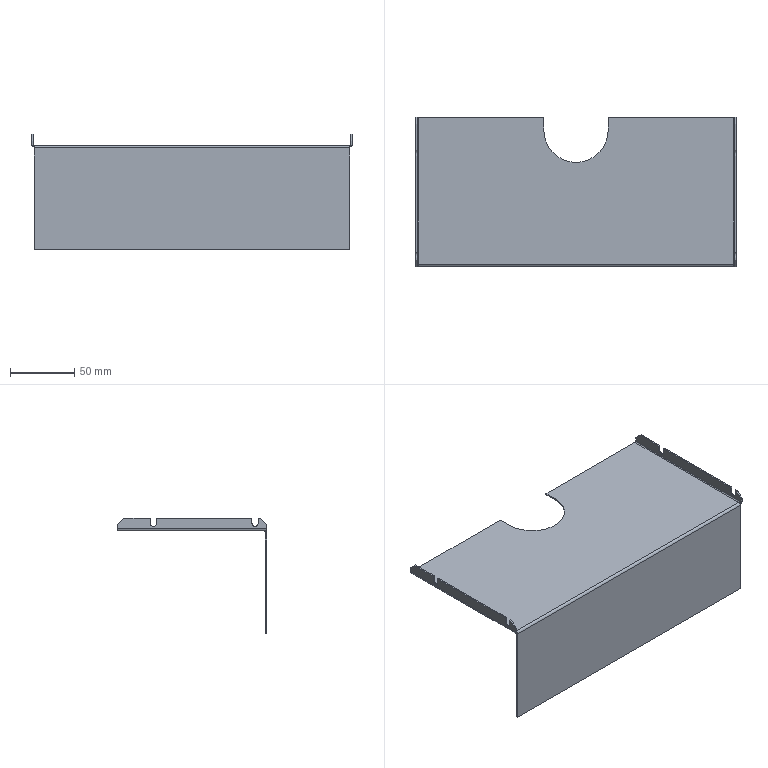Part | SolidWorks | features EdgeFlange 2, BreakCorner 1, FlatPattern 1, HoleWzd 1, ICE 1, MoveFace 1, SMBaseFlange 1, SheetMetal 1 | 1 solid | 60 faces | box 249 x 116 x 90 mm | volume 48716 mm3 | plane 45 | cylinder 15 | commonest cylinder face diameters 4.8 x8 1.473 x3 3.473 x3 50 x1